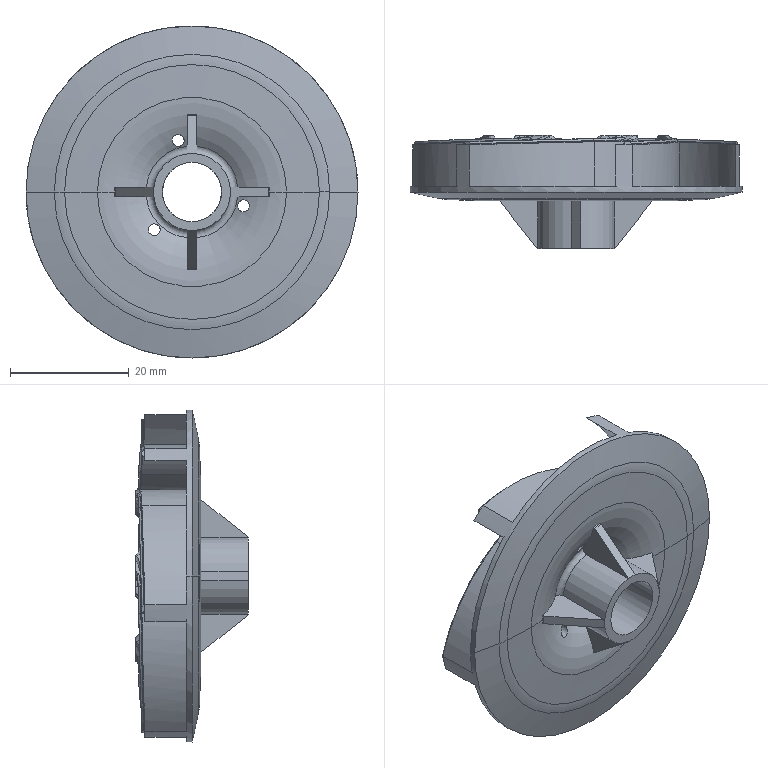Part | STEP file | DW-T1-02-0033_2_6_1 | 1 solid | 222 faces | box 56 x 19.052 x 56 mm | volume 7855 mm3 | cylinder 80 | spline 60 | torus 30 | cone 28 | plane 24 | commonest cylinder face diameters 2 x6 18.4 x6 21.2 x6 35.2 x6 35.9 x6 37.3 x6